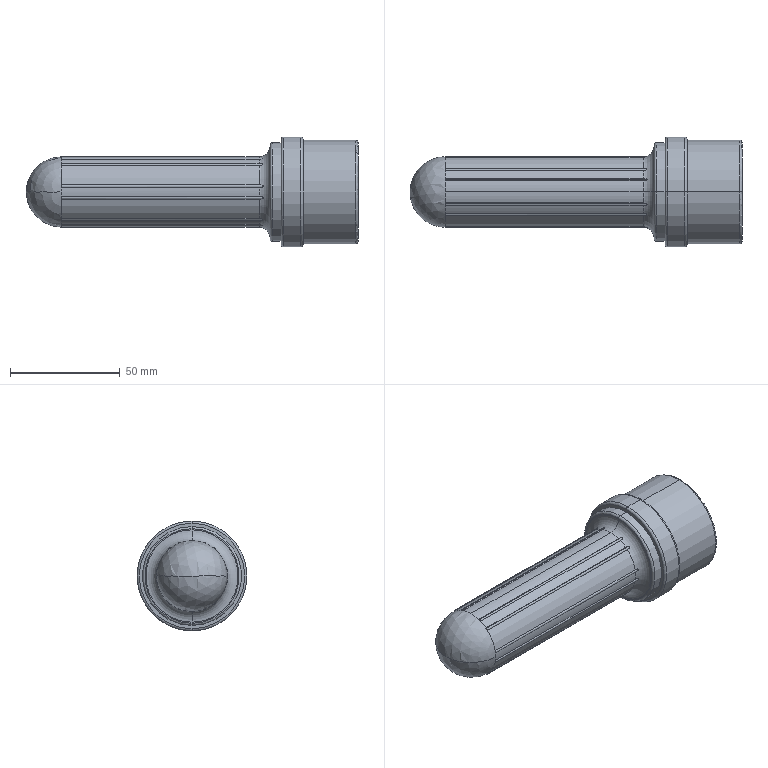Part | NX | features BREP 1 | 1 solid | 71 faces | box 151 x 50 x 50 mm | volume 105394 mm3 | cylinder 37 | plane 18 | torus 10 | cone 4 | sphere 2 | commonest cylinder face diameters 1.414 x16 32 x13 22 x2 45 x2 47 x2 50 x2